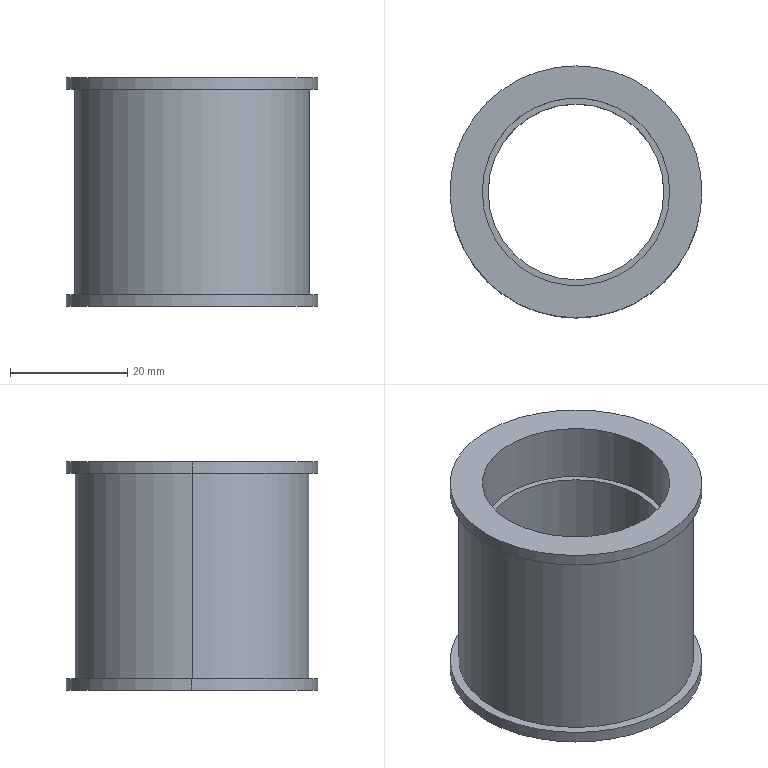Part | STEP file | Driven wheel | 1 solid | 18 faces | box 43 x 43 x 39 mm | volume 20276 mm3 | cylinder 12 | plane 6 | commonest cylinder face diameters 32 x4 43 x4 30 x2 40 x2
STEP:
#1=CARTESIAN_POINT('',(0.,0.,0.));
#2=DIRECTION('',(0.,0.,1.));
#3=DIRECTION('',(1.,0.,0.));
#4=AXIS2_PLACEMENT_3D('',#1,#2,#3);
#5=CARTESIAN_POINT('',(-20.,0.,35.));
#6=VERTEX_POINT('',#5);
#7=CARTESIAN_POINT('',(20.,0.,35.));
#8=VERTEX_POINT('',#7);
#9=CARTESIAN_POINT('',(0.,0.,35.));
#10=DIRECTION('',(0.,0.,-1.));
#11=DIRECTION('',(-1.,0.,0.));
#12=AXIS2_PLACEMENT_3D('',#9,#10,#11);
#13=CIRCLE('',#12,20.);
#14=CARTESIAN_POINT('',(0.,0.,35.));
#15=DIRECTION('',(0.,0.,-1.));
#16=DIRECTION('',(-1.,0.,0.));
#17=AXIS2_PLACEMENT_3D('',#14,#15,#16);
#18=CYLINDRICAL_SURFACE('',#17,20.);
#19=CARTESIAN_POINT('',(0.,0.));
#20=DIRECTION('',(1.,0.));
#21=VECTOR('',#20,1.);
#22=LINE('',#19,#21);
#23=(GEOMETRIC_REPRESENTATION_CONTEXT(2)PARAMETRIC_REPRESENTATION_CONTEXT()REPRESENTATION_CONTEXT('',''));
#24=DEFINITIONAL_REPRESENTATION('',(#22),#23);
#25=PCURVE('',#18,#24);
#26=CARTESIAN_POINT('',(0.,0.,35.));
#27=DIRECTION('',(0.,0.,1.));
#28=DIRECTION('',(1.,0.,0.));
#29=AXIS2_PLACEMENT_3D('',#26,#27,#28);
#30=PLANE('',#29);
#31=CARTESIAN_POINT('',(-20.,0.));
#32=CARTESIAN_POINT('',(-20.,34.641));
#33=CARTESIAN_POINT('',(10.,17.321));
#34=CARTESIAN_POINT('',(40.,0.));
#35=CARTESIAN_POINT('',(10.,-17.321));
#36=CARTESIAN_POINT('',(-20.,-34.641));
#37=CARTESIAN_POINT('',(-20.,0.));
#38=(BOUNDED_CURVE()B_SPLINE_CURVE(2,(#31,#32,#33,#34,#35,#36,#37),.UNSPECIFIED.,.T.,.F.)B_SPLINE_CURVE_WITH_KNOTS((1,2,2,2,2,1),(-2.094,0.,2.094,4.189,6.283,8.378),.UNSPECIFIED.)CURVE()GEOMETRIC_REPRESENTATION_ITEM()RATIONAL_B_SPLINE_CURVE((1.,0.5,1.,0.5,1.,0.5,1.))REPRESENTATION_ITEM(''));
#39=(GEOMETRIC_REPRESENTATION_CONTEXT(2)PARAMETRIC_REPRESENTATION_CONTEXT()REPRESENTATION_CONTEXT('',''));
#40=DEFINITIONAL_REPRESENTATION('',(#38),#39);
#41=PCURVE('',#30,#40);
#42=SURFACE_CURVE('',#13,(#25,#41),.PCURVE_S1.);
#43=EDGE_CURVE('',#6,#8,#42,.T.);
#44=ORIENTED_EDGE('',*,*,#43,.T.);
#45=CARTESIAN_POINT('',(20.,0.,0.));
#46=VERTEX_POINT('',#45);
#47=CARTESIAN_POINT('',(20.,0.,35.));
#48=DIRECTION('',(0.,0.,-1.));
#49=VECTOR('',#48,1.);
#50=LINE('',#47,#49);
#51=CARTESIAN_POINT('',(3.142,0.));
#52=DIRECTION('',(0.,1.));
#53=VECTOR('',#52,1.);
#54=LINE('',#51,#53);
#55=(GEOMETRIC_REPRESENTATION_CONTEXT(2)PARAMETRIC_REPRESENTATION_CONTEXT()REPRESENTATION_CONTEXT('',''));
#56=DEFINITIONAL_REPRESENTATION('',(#54),#55);
#57=PCURVE('',#18,#56);
#58=CARTESIAN_POINT('',(0.,0.,35.));
#59=DIRECTION('',(0.,0.,-1.));
#60=DIRECTION('',(-1.,0.,0.));
#61=AXIS2_PLACEMENT_3D('',#58,#59,#60);
#62=CYLINDRICAL_SURFACE('',#61,20.);
#63=CARTESIAN_POINT('',(3.142,0.));
#64=DIRECTION('',(0.,1.));
#65=VECTOR('',#64,1.);
#66=LINE('',#63,#65);
#67=(GEOMETRIC_REPRESENTATION_CONTEXT(2)PARAMETRIC_REPRESENTATION_CONTEXT()REPRESENTATION_CONTEXT('',''));
#68=DEFINITIONAL_REPRESENTATION('',(#66),#67);
#69=PCURVE('',#62,#68);
#70=SURFACE_CURVE('',#50,(#57,#69),.PCURVE_S1.);
#71=EDGE_CURVE('',#8,#46,#70,.T.);
#72=ORIENTED_EDGE('',*,*,#71,.T.);
#73=CARTESIAN_POINT('',(-20.,0.,0.));
#74=VERTEX_POINT('',#73);
#75=CARTESIAN_POINT('',(0.,0.,0.));
#76=DIRECTION('',(0.,0.,1.));
#77=DIRECTION('',(-1.,0.,0.));
#78=AXIS2_PLACEMENT_3D('',#75,#76,#77);
#79=CIRCLE('',#78,20.);
#80=CARTESIAN_POINT('',(6.283,35.));
#81=DIRECTION('',(-1.,0.));
#82=VECTOR('',#81,1.);
#83=LINE('',#80,#82);
#84=(GEOMETRIC_REPRESENTATION_CONTEXT(2)PARAMETRIC_REPRESENTATION_CONTEXT()REPRESENTATION_CONTEXT('',''));
#85=DEFINITIONAL_REPRESENTATION('',(#83),#84);
#86=PCURVE('',#18,#85);
#87=CARTESIAN_POINT('',(0.,0.,0.));
#88=DIRECTION('',(0.,0.,-1.));
#89=DIRECTION('',(-1.,0.,0.));
#90=AXIS2_PLACEMENT_3D('',#87,#88,#89);
#91=PLANE('',#90);
#92=CARTESIAN_POINT('',(20.,0.));
#93=CARTESIAN_POINT('',(20.,-34.641));
#94=CARTESIAN_POINT('',(-10.,-17.321));
#95=CARTESIAN_POINT('',(-40.,0.));
#96=CARTESIAN_POINT('',(-10.,17.321));
#97=CARTESIAN_POINT('',(20.,34.641));
#98=CARTESIAN_POINT('',(20.,0.));
#99=(BOUNDED_CURVE()B_SPLINE_CURVE(2,(#92,#93,#94,#95,#96,#97,#98),.UNSPECIFIED.,.T.,.F.)B_SPLINE_CURVE_WITH_KNOTS((1,2,2,2,2,1),(-2.094,0.,2.094,4.189,6.283,8.378),.UNSPECIFIED.)CURVE()GEOMETRIC_REPRESENTATION_ITEM()RATIONAL_B_SPLINE_CURVE((1.,0.5,1.,0.5,1.,0.5,1.))REPRESENTATION_ITEM(''));
#100=(GEOMETRIC_REPRESENTATION_CONTEXT(2)PARAMETRIC_REPRESENTATION_CONTEXT()REPRESENTATION_CONTEXT('',''));
#101=DEFINITIONAL_REPRESENTATION('',(#99),#100);
#102=PCURVE('',#91,#101);
#103=SURFACE_CURVE('',#79,(#86,#102),.PCURVE_S1.);
#104=EDGE_CURVE('',#46,#74,#103,.T.);
#105=ORIENTED_EDGE('',*,*,#104,.T.);
#106=CARTESIAN_POINT('',(-20.,0.,35.));
#107=DIRECTION('',(0.,0.,-1.));
#108=VECTOR('',#107,1.);
#109=LINE('',#106,#108);
#110=CARTESIAN_POINT('',(0.,0.));
#111=DIRECTION('',(0.,1.));
#112=VECTOR('',#111,1.);
#113=LINE('',#110,#112);
#114=(GEOMETRIC_REPRESENTATION_CONTEXT(2)PARAMETRIC_REPRESENTATION_CONTEXT()REPRESENTATION_CONTEXT('',''));
#115=DEFINITIONAL_REPRESENTATION('',(#113),#114);
#116=PCURVE('',#18,#115);
#117=CARTESIAN_POINT('',(6.283,0.));
#118=DIRECTION('',(0.,1.));
#119=VECTOR('',#118,1.);
#120=LINE('',#117,#119);
#121=(GEOMETRIC_REPRESENTATION_CONTEXT(2)PARAMETRIC_REPRESENTATION_CONTEXT()REPRESENTATION_CONTEXT('',''));
#122=DEFINITIONAL_REPRESENTATION('',(#120),#121);
#123=PCURVE('',#62,#122);
#124=SURFACE_CURVE('',#109,(#116,#123),.PCURVE_S1.);
#125=EDGE_CURVE('',#6,#74,#124,.T.);
#126=ORIENTED_EDGE('',*,*,#125,.F.);
#127=EDGE_LOOP('',(#44,#72,#105,#126));
#128=FACE_BOUND('',#127,.T.);
#129=ADVANCED_FACE('',(#128),#18,.T.);
#130=CARTESIAN_POINT('',(21.5,0.,-2.));
#131=VERTEX_POINT('',#130);
#132=CARTESIAN_POINT('',(-21.5,0.,-2.));
#133=VERTEX_POINT('',#132);
#134=CARTESIAN_POINT('',(0.,0.,-2.));
#135=DIRECTION('',(0.,0.,1.));
#136=DIRECTION('',(1.,0.,0.));
#137=AXIS2_PLACEMENT_3D('',#134,#135,#136);
#138=CIRCLE('',#137,21.5);
#139=CARTESIAN_POINT('',(0.,0.,-2.));
#140=DIRECTION('',(0.,0.,1.));
#141=DIRECTION('',(1.,0.,0.));
#142=AXIS2_PLACEMENT_3D('',#139,#140,#141);
#143=CYLINDRICAL_SURFACE('',#142,21.5);
#144=CARTESIAN_POINT('',(0.,0.));
#145=DIRECTION('',(1.,0.));
#146=VECTOR('',#145,1.);
#147=LINE('',#144,#146);
#148=(GEOMETRIC_REPRESENTATION_CONTEXT(2)PARAMETRIC_REPRESENTATION_CONTEXT()REPRESENTATION_CONTEXT('',''));
#149=DEFINITIONAL_REPRESENTATION('',(#147),#148);
#150=PCURVE('',#143,#149);
#151=CARTESIAN_POINT('',(0.,0.,-2.));
#152=DIRECTION('',(0.,0.,-1.));
#153=DIRECTION('',(-1.,0.,0.));
#154=AXIS2_PLACEMENT_3D('',#151,#152,#153);
#155=PLANE('',#154);
#156=CARTESIAN_POINT('',(-21.5,0.));
#157=CARTESIAN_POINT('',(-21.5,37.239));
#158=CARTESIAN_POINT('',(10.75,18.62));
#159=CARTESIAN_POINT('',(43.,0.));
#160=CARTESIAN_POINT('',(10.75,-18.62));
#161=CARTESIAN_POINT('',(-21.5,-37.239));
#162=CARTESIAN_POINT('',(-21.5,0.));
#163=(BOUNDED_CURVE()B_SPLINE_CURVE(2,(#156,#157,#158,#159,#160,#161,#162),.UNSPECIFIED.,.T.,.F.)B_SPLINE_CURVE_WITH_KNOTS((1,2,2,2,2,1),(-2.094,0.,2.094,4.189,6.283,8.378),.UNSPECIFIED.)CURVE()GEOMETRIC_REPRESENTATION_ITEM()RATIONAL_B_SPLINE_CURVE((1.,0.5,1.,0.5,1.,0.5,1.))REPRESENTATION_ITEM(''));
#164=(GEOMETRIC_REPRESENTATION_CONTEXT(2)PARAMETRIC_REPRESENTATION_CONTEXT()REPRESENTATION_CONTEXT('',''));
#165=DEFINITIONAL_REPRESENTATION('',(#163),#164);
#166=PCURVE('',#155,#165);
#167=SURFACE_CURVE('',#138,(#150,#166),.PCURVE_S1.);
#168=EDGE_CURVE('',#131,#133,#167,.T.);
#169=ORIENTED_EDGE('',*,*,#168,.T.);
#170=CARTESIAN_POINT('',(-21.5,0.,0.));
#171=VERTEX_POINT('',#170);
#172=CARTESIAN_POINT('',(-21.5,0.,-2.));
#173=DIRECTION('',(0.,0.,1.));
#174=VECTOR('',#173,1.);
#175=LINE('',#172,#174);
#176=CARTESIAN_POINT('',(3.142,0.));
#177=DIRECTION('',(0.,1.));
#178=VECTOR('',#177,1.);
#179=LINE('',#176,#178);
#180=(GEOMETRIC_REPRESENTATION_CONTEXT(2)PARAMETRIC_REPRESENTATION_CONTEXT()REPRESENTATION_CONTEXT('',''));
#181=DEFINITIONAL_REPRESENTATION('',(#179),#180);
#182=PCURVE('',#143,#181);
#183=CARTESIAN_POINT('',(0.,0.,-2.));
#184=DIRECTION('',(0.,0.,1.));
#185=DIRECTION('',(1.,0.,0.));
#186=AXIS2_PLACEMENT_3D('',#183,#184,#185);
#187=CYLINDRICAL_SURFACE('',#186,21.5);
#188=CARTESIAN_POINT('',(3.142,0.));
#189=DIRECTION('',(0.,1.));
#190=VECTOR('',#189,1.);
#191=LINE('',#188,#190);
#192=(GEOMETRIC_REPRESENTATION_CONTEXT(2)PARAMETRIC_REPRESENTATION_CONTEXT()REPRESENTATION_CONTEXT('',''));
#193=DEFINITIONAL_REPRESENTATION('',(#191),#192);
#194=PCURVE('',#187,#193);
#195=SURFACE_CURVE('',#175,(#182,#194),.PCURVE_S1.);
#196=EDGE_CURVE('',#133,#171,#195,.T.);
#197=ORIENTED_EDGE('',*,*,#196,.T.);
#198=CARTESIAN_POINT('',(21.5,0.,0.));
#199=VERTEX_POINT('',#198);
#200=CARTESIAN_POINT('',(0.,0.,0.));
#201=DIRECTION('',(0.,0.,-1.));
#202=DIRECTION('',(1.,0.,0.));
#203=AXIS2_PLACEMENT_3D('',#200,#201,#202);
#204=CIRCLE('',#203,21.5);
#205=CARTESIAN_POINT('',(6.283,2.));
#206=DIRECTION('',(-1.,0.));
#207=VECTOR('',#206,1.);
#208=LINE('',#205,#207);
#209=(GEOMETRIC_REPRESENTATION_CONTEXT(2)PARAMETRIC_REPRESENTATION_CONTEXT()REPRESENTATION_CONTEXT('',''));
#210=DEFINITIONAL_REPRESENTATION('',(#208),#209);
#211=PCURVE('',#143,#210);
#212=CARTESIAN_POINT('',(0.,0.));
#213=DIRECTION('',(-1.,0.));
#214=AXIS2_PLACEMENT_2D('',#212,#213);
#215=CIRCLE('',#214,21.5);
#216=(GEOMETRIC_REPRESENTATION_CONTEXT(2)PARAMETRIC_REPRESENTATION_CONTEXT()REPRESENTATION_CONTEXT('',''));
#217=DEFINITIONAL_REPRESENTATION('',(#215),#216);
#218=PCURVE('',#91,#217);
#219=SURFACE_CURVE('',#204,(#211,#218),.PCURVE_S1.);
#220=EDGE_CURVE('',#171,#199,#219,.T.);
#221=ORIENTED_EDGE('',*,*,#220,.T.);
#222=CARTESIAN_POINT('',(21.5,0.,-2.));
#223=DIRECTION('',(0.,0.,1.));
#224=VECTOR('',#223,1.);
#225=LINE('',#222,#224);
#226=CARTESIAN_POINT('',(0.,0.));
#227=DIRECTION('',(0.,1.));
#228=VECTOR('',#227,1.);
#229=LINE('',#226,#228);
#230=(GEOMETRIC_REPRESENTATION_CONTEXT(2)PARAMETRIC_REPRESENTATION_CONTEXT()REPRESENTATION_CONTEXT('',''));
#231=DEFINITIONAL_REPRESENTATION('',(#229),#230);
#232=PCURVE('',#143,#231);
#233=CARTESIAN_POINT('',(6.283,0.));
#234=DIRECTION('',(0.,1.));
#235=VECTOR('',#234,1.);
#236=LINE('',#233,#235);
#237=(GEOMETRIC_REPRESENTATION_CONTEXT(2)PARAMETRIC_REPRESENTATION_CONTEXT()REPRESENTATION_CONTEXT('',''));
#238=DEFINITIONAL_REPRESENTATION('',(#236),#237);
#239=PCURVE('',#187,#238);
#240=SURFACE_CURVE('',#225,(#232,#239),.PCURVE_S1.);
#241=EDGE_CURVE('',#131,#199,#240,.T.);
#242=ORIENTED_EDGE('',*,*,#241,.F.);
#243=EDGE_LOOP('',(#169,#197,#221,#242));
#244=FACE_BOUND('',#243,.T.);
#245=ADVANCED_FACE('',(#244),#143,.T.);
#246=CARTESIAN_POINT('',(-21.5,0.,37.));
#247=VERTEX_POINT('',#246);
#248=CARTESIAN_POINT('',(21.5,0.,37.));
#249=VERTEX_POINT('',#248);
#250=CARTESIAN_POINT('',(0.,0.,37.));
#251=DIRECTION('',(0.,0.,-1.));
#252=DIRECTION('',(-1.,0.,0.));
#253=AXIS2_PLACEMENT_3D('',#250,#251,#252);
#254=CIRCLE('',#253,21.5);
#255=CARTESIAN_POINT('',(0.,0.,37.));
#256=DIRECTION('',(0.,0.,-1.));
#257=DIRECTION('',(-1.,0.,0.));
#258=AXIS2_PLACEMENT_3D('',#255,#256,#257);
#259=CYLINDRICAL_SURFACE('',#258,21.5);
#260=CARTESIAN_POINT('',(0.,0.));
#261=DIRECTION('',(1.,0.));
#262=VECTOR('',#261,1.);
#263=LINE('',#260,#262);
#264=(GEOMETRIC_REPRESENTATION_CONTEXT(2)PARAMETRIC_REPRESENTATION_CONTEXT()REPRESENTATION_CONTEXT('',''));
#265=DEFINITIONAL_REPRESENTATION('',(#263),#264);
#266=PCURVE('',#259,#265);
#267=CARTESIAN_POINT('',(0.,0.,37.));
#268=DIRECTION('',(0.,0.,1.));
#269=DIRECTION('',(1.,0.,0.));
#270=AXIS2_PLACEMENT_3D('',#267,#268,#269);
#271=PLANE('',#270);
#272=CARTESIAN_POINT('',(-21.5,0.));
#273=CARTESIAN_POINT('',(-21.5,37.239));
#274=CARTESIAN_POINT('',(10.75,18.62));
#275=CARTESIAN_POINT('',(43.,0.));
#276=CARTESIAN_POINT('',(10.75,-18.62));
#277=CARTESIAN_POINT('',(-21.5,-37.239));
#278=CARTESIAN_POINT('',(-21.5,0.));
#279=(BOUNDED_CURVE()B_SPLINE_CURVE(2,(#272,#273,#274,#275,#276,#277,#278),.UNSPECIFIED.,.T.,.F.)B_SPLINE_CURVE_WITH_KNOTS((1,2,2,2,2,1),(-2.094,0.,2.094,4.189,6.283,8.378),.UNSPECIFIED.)CURVE()GEOMETRIC_REPRESENTATION_ITEM()RATIONAL_B_SPLINE_CURVE((1.,0.5,1.,0.5,1.,0.5,1.))REPRESENTATION_ITEM(''));
#280=(GEOMETRIC_REPRESENTATION_CONTEXT(2)PARAMETRIC_REPRESENTATION_CONTEXT()REPRESENTATION_CONTEXT('',''));
#281=DEFINITIONAL_REPRESENTATION('',(#279),#280);
#282=PCURVE('',#271,#281);
#283=SURFACE_CURVE('',#254,(#266,#282),.PCURVE_S1.);
#284=EDGE_CURVE('',#247,#249,#283,.T.);
#285=ORIENTED_EDGE('',*,*,#284,.T.);
#286=CARTESIAN_POINT('',(21.5,0.,35.));
#287=VERTEX_POINT('',#286);
#288=CARTESIAN_POINT('',(21.5,0.,37.));
#289=DIRECTION('',(0.,0.,-1.));
#290=VECTOR('',#289,1.);
#291=LINE('',#288,#290);
#292=CARTESIAN_POINT('',(3.142,0.));
#293=DIRECTION('',(0.,1.));
#294=VECTOR('',#293,1.);
#295=LINE('',#292,#294);
#296=(GEOMETRIC_REPRESENTATION_CONTEXT(2)PARAMETRIC_REPRESENTATION_CONTEXT()REPRESENTATION_CONTEXT('',''));
#297=DEFINITIONAL_REPRESENTATION('',(#295),#296);
#298=PCURVE('',#259,#297);
#299=CARTESIAN_POINT('',(0.,0.,37.));
#300=DIRECTION('',(0.,0.,-1.));
#301=DIRECTION('',(-1.,0.,0.));
#302=AXIS2_PLACEMENT_3D('',#299,#300,#301);
#303=CYLINDRICAL_SURFACE('',#302,21.5);
#304=CARTESIAN_POINT('',(3.142,0.));
#305=DIRECTION('',(0.,1.));
#306=VECTOR('',#305,1.);
#307=LINE('',#304,#306);
#308=(GEOMETRIC_REPRESENTATION_CONTEXT(2)PARAMETRIC_REPRESENTATION_CONTEXT()REPRESENTATION_CONTEXT('',''));
#309=DEFINITIONAL_REPRESENTATION('',(#307),#308);
#310=PCURVE('',#303,#309);
#311=SURFACE_CURVE('',#291,(#298,#310),.PCURVE_S1.);
#312=EDGE_CURVE('',#249,#287,#311,.T.);
#313=ORIENTED_EDGE('',*,*,#312,.T.);
#314=CARTESIAN_POINT('',(-21.5,0.,35.));
#315=VERTEX_POINT('',#314);
#316=CARTESIAN_POINT('',(0.,0.,35.));
#317=DIRECTION('',(0.,0.,1.));
#318=DIRECTION('',(-1.,0.,0.));
#319=AXIS2_PLACEMENT_3D('',#316,#317,#318);
#320=CIRCLE('',#319,21.5);
#321=CARTESIAN_POINT('',(6.283,2.));
#322=DIRECTION('',(-1.,0.));
#323=VECTOR('',#322,1.);
#324=LINE('',#321,#323);
#325=(GEOMETRIC_REPRESENTATION_CONTEXT(2)PARAMETRIC_REPRESENTATION_CONTEXT()REPRESENTATION_CONTEXT('',''));
#326=DEFINITIONAL_REPRESENTATION('',(#324),#325);
#327=PCURVE('',#259,#326);
#328=CARTESIAN_POINT('',(0.,0.));
#329=DIRECTION('',(-1.,0.));
#330=AXIS2_PLACEMENT_2D('',#328,#329);
#331=CIRCLE('',#330,21.5);
#332=(GEOMETRIC_REPRESENTATION_CONTEXT(2)PARAMETRIC_REPRESENTATION_CONTEXT()REPRESENTATION_CONTEXT('',''));
#333=DEFINITIONAL_REPRESENTATION('',(#331),#332);
#334=PCURVE('',#30,#333);
#335=SURFACE_CURVE('',#320,(#327,#334),.PCURVE_S1.);
#336=EDGE_CURVE('',#287,#315,#335,.T.);
#337=ORIENTED_EDGE('',*,*,#336,.T.);
#338=CARTESIAN_POINT('',(-21.5,0.,37.));
#339=DIRECTION('',(0.,0.,-1.));
#340=VECTOR('',#339,1.);
#341=LINE('',#338,#340);
#342=CARTESIAN_POINT('',(0.,0.));
#343=DIRECTION('',(0.,1.));
#344=VECTOR('',#343,1.);
#345=LINE('',#342,#344);
#346=(GEOMETRIC_REPRESENTATION_CONTEXT(2)PARAMETRIC_REPRESENTATION_CONTEXT()REPRESENTATION_CONTEXT('',''));
#347=DEFINITIONAL_REPRESENTATION('',(#345),#346);
#348=PCURVE('',#259,#347);
#349=CARTESIAN_POINT('',(6.283,0.));
#350=DIRECTION('',(0.,1.));
#351=VECTOR('',#350,1.);
#352=LINE('',#349,#351);
#353=(GEOMETRIC_REPRESENTATION_CONTEXT(2)PARAMETRIC_REPRESENTATION_CONTEXT()REPRESENTATION_CONTEXT('',''));
#354=DEFINITIONAL_REPRESENTATION('',(#352),#353);
#355=PCURVE('',#303,#354);
#356=SURFACE_CURVE('',#341,(#348,#355),.PCURVE_S1.);
#357=EDGE_CURVE('',#247,#315,#356,.T.);
#358=ORIENTED_EDGE('',*,*,#357,.F.);
#359=EDGE_LOOP('',(#285,#313,#337,#358));
#360=FACE_BOUND('',#359,.T.);
#361=ADVANCED_FACE('',(#360),#259,.T.);
#362=CARTESIAN_POINT('',(-16.,0.,8.));
#363=VERTEX_POINT('',#362);
#364=CARTESIAN_POINT('',(-16.,0.,-2.));
#365=VERTEX_POINT('',#364);
#366=CARTESIAN_POINT('',(-16.,0.,8.));
#367=DIRECTION('',(0.,0.,-1.));
#368=VECTOR('',#367,1.);
#369=LINE('',#366,#368);
#370=CARTESIAN_POINT('',(0.,0.,8.));
#371=DIRECTION('',(0.,0.,-1.));
#372=DIRECTION('',(-1.,0.,0.));
#373=AXIS2_PLACEMENT_3D('',#370,#371,#372);
#374=CYLINDRICAL_SURFACE('',#373,16.);
#375=CARTESIAN_POINT('',(6.283,0.));
#376=DIRECTION('',(0.,1.));
#377=VECTOR('',#376,1.);
#378=LINE('',#375,#377);
#379=(GEOMETRIC_REPRESENTATION_CONTEXT(2)PARAMETRIC_REPRESENTATION_CONTEXT()REPRESENTATION_CONTEXT('',''));
#380=DEFINITIONAL_REPRESENTATION('',(#378),#379);
#381=PCURVE('',#374,#380);
#382=CARTESIAN_POINT('',(0.,0.,8.));
#383=DIRECTION('',(0.,0.,-1.));
#384=DIRECTION('',(-1.,0.,0.));
#385=AXIS2_PLACEMENT_3D('',#382,#383,#384);
#386=CYLINDRICAL_SURFACE('',#385,16.);
#387=CARTESIAN_POINT('',(0.,0.));
#388=DIRECTION('',(0.,1.));
#389=VECTOR('',#388,1.);
#390=LINE('',#387,#389);
#391=(GEOMETRIC_REPRESENTATION_CONTEXT(2)PARAMETRIC_REPRESENTATION_CONTEXT()REPRESENTATION_CONTEXT('',''));
#392=DEFINITIONAL_REPRESENTATION('',(#390),#391);
#393=PCURVE('',#386,#392);
#394=SURFACE_CURVE('',#369,(#381,#393),.PCURVE_S1.);
#395=EDGE_CURVE('',#363,#365,#394,.T.);
#396=ORIENTED_EDGE('',*,*,#395,.T.);
#397=CARTESIAN_POINT('',(16.,0.,-2.));
#398=VERTEX_POINT('',#397);
#399=CARTESIAN_POINT('',(0.,0.,-2.));
#400=DIRECTION('',(0.,0.,1.));
#401=DIRECTION('',(-1.,0.,0.));
#402=AXIS2_PLACEMENT_3D('',#399,#400,#401);
#403=CIRCLE('',#402,16.);
#404=CARTESIAN_POINT('',(6.283,10.));
#405=DIRECTION('',(-1.,0.));
#406=VECTOR('',#405,1.);
#407=LINE('',#404,#406);
#408=(GEOMETRIC_REPRESENTATION_CONTEXT(2)PARAMETRIC_REPRESENTATION_CONTEXT()REPRESENTATION_CONTEXT('',''));
#409=DEFINITIONAL_REPRESENTATION('',(#407),#408);
#410=PCURVE('',#374,#409);
#411=CARTESIAN_POINT('',(16.,0.));
#412=CARTESIAN_POINT('',(16.,-27.713));
#413=CARTESIAN_POINT('',(-8.,-13.856));
#414=CARTESIAN_POINT('',(-32.,0.));
#415=CARTESIAN_POINT('',(-8.,13.856));
#416=CARTESIAN_POINT('',(16.,27.713));
#417=CARTESIAN_POINT('',(16.,0.));
#418=(BOUNDED_CURVE()B_SPLINE_CURVE(2,(#411,#412,#413,#414,#415,#416,#417),.UNSPECIFIED.,.T.,.F.)B_SPLINE_CURVE_WITH_KNOTS((1,2,2,2,2,1),(-2.094,0.,2.094,4.189,6.283,8.378),.UNSPECIFIED.)CURVE()GEOMETRIC_REPRESENTATION_ITEM()RATIONAL_B_SPLINE_CURVE((1.,0.5,1.,0.5,1.,0.5,1.))REPRESENTATION_ITEM(''));
#419=(GEOMETRIC_REPRESENTATION_CONTEXT(2)PARAMETRIC_REPRESENTATION_CONTEXT()REPRESENTATION_CONTEXT('',''));
#420=DEFINITIONAL_REPRESENTATION('',(#418),#419);
#421=PCURVE('',#155,#420);
#422=SURFACE_CURVE('',#403,(#410,#421),.PCURVE_S1.);
#423=EDGE_CURVE('',#365,#398,#422,.T.);
#424=ORIENTED_EDGE('',*,*,#423,.T.);
#425=CARTESIAN_POINT('',(16.,0.,8.));
#426=VERTEX_POINT('',#425);
#427=CARTESIAN_POINT('',(16.,0.,8.));
#428=DIRECTION('',(0.,0.,-1.));
#429=VECTOR('',#428,1.);
#430=LINE('',#427,#429);
#431=CARTESIAN_POINT('',(3.142,0.));
#432=DIRECTION('',(0.,1.));
#433=VECTOR('',#432,1.);
#434=LINE('',#431,#433);
#435=(GEOMETRIC_REPRESENTATION_CONTEXT(2)PARAMETRIC_REPRESENTATION_CONTEXT()REPRESENTATION_CONTEXT('',''));
#436=DEFINITIONAL_REPRESENTATION('',(#434),#435);
#437=PCURVE('',#374,#436);
#438=CARTESIAN_POINT('',(3.142,0.));
#439=DIRECTION('',(0.,1.));
#440=VECTOR('',#439,1.);
#441=LINE('',#438,#440);
#442=(GEOMETRIC_REPRESENTATION_CONTEXT(2)PARAMETRIC_REPRESENTATION_CONTEXT()REPRESENTATION_CONTEXT('',''));
#443=DEFINITIONAL_REPRESENTATION('',(#441),#442);
#444=PCURVE('',#386,#443);
#445=SURFACE_CURVE('',#430,(#437,#444),.PCURVE_S1.);
#446=EDGE_CURVE('',#426,#398,#445,.T.);
#447=ORIENTED_EDGE('',*,*,#446,.F.);
#448=CARTESIAN_POINT('',(0.,0.,8.));
#449=DIRECTION('',(0.,0.,-1.));
#450=DIRECTION('',(-1.,0.,0.));
#451=AXIS2_PLACEMENT_3D('',#448,#449,#450);
#452=CIRCLE('',#451,16.);
#453=CARTESIAN_POINT('',(0.,0.));
#454=DIRECTION('',(1.,0.));
#455=VECTOR('',#454,1.);
#456=LINE('',#453,#455);
#457=(GEOMETRIC_REPRESENTATION_CONTEXT(2)PARAMETRIC_REPRESENTATION_CONTEXT()REPRESENTATION_CONTEXT('',''));
#458=DEFINITIONAL_REPRESENTATION('',(#456),#457);
#459=PCURVE('',#374,#458);
#460=CARTESIAN_POINT('',(0.,0.,8.));
#461=DIRECTION('',(0.,0.,-1.));
#462=DIRECTION('',(-1.,0.,0.));
#463=AXIS2_PLACEMENT_3D('',#460,#461,#462);
#464=PLANE('',#463);
#465=CARTESIAN_POINT('',(0.,0.));
#466=DIRECTION('',(1.,0.));
#467=AXIS2_PLACEMENT_2D('',#465,#466);
#468=CIRCLE('',#467,16.);
#469=(GEOMETRIC_REPRESENTATION_CONTEXT(2)PARAMETRIC_REPRESENTATION_CONTEXT()REPRESENTATION_CONTEXT('',''));
#470=DEFINITIONAL_REPRESENTATION('',(#468),#469);
#471=PCURVE('',#464,#470);
#472=SURFACE_CURVE('',#452,(#459,#471),.PCURVE_S1.);
#473=EDGE_CURVE('',#426,#363,#472,.T.);
#474=ORIENTED_EDGE('',*,*,#473,.T.);
#475=EDGE_LOOP('',(#396,#424,#447,#474));
#476=FACE_BOUND('',#475,.F.);
#477=ADVANCED_FACE('',(#476),#374,.F.);
#478=CARTESIAN_POINT('',(16.,0.,27.));
#479=VERTEX_POINT('',#478);
#480=CARTESIAN_POINT('',(16.,0.,37.));
#481=VERTEX_POINT('',#480);
#482=CARTESIAN_POINT('',(16.,0.,27.));
#483=DIRECTION('',(0.,0.,1.));
#484=VECTOR('',#483,1.);
#485=LINE('',#482,#484);
#486=CARTESIAN_POINT('',(0.,0.,27.));
#487=DIRECTION('',(0.,0.,1.));
#488=DIRECTION('',(1.,0.,0.));
#489=AXIS2_PLACEMENT_3D('',#486,#487,#488);
#490=CYLINDRICAL_SURFACE('',#489,16.);
#491=CARTESIAN_POINT('',(6.283,0.));
#492=DIRECTION('',(0.,1.));
#493=VECTOR('',#492,1.);
#494=LINE('',#491,#493);
#495=(GEOMETRIC_REPRESENTATION_CONTEXT(2)PARAMETRIC_REPRESENTATION_CONTEXT()REPRESENTATION_CONTEXT('',''));
#496=DEFINITIONAL_REPRESENTATION('',(#494),#495);
#497=PCURVE('',#490,#496);
#498=CARTESIAN_POINT('',(0.,0.,27.));
#499=DIRECTION('',(0.,0.,1.));
#500=DIRECTION('',(1.,0.,0.));
#501=AXIS2_PLACEMENT_3D('',#498,#499,#500);
#502=CYLINDRICAL_SURFACE('',#501,16.);
#503=CARTESIAN_POINT('',(0.,0.));
#504=DIRECTION('',(0.,1.));
#505=VECTOR('',#504,1.);
#506=LINE('',#503,#505);
#507=(GEOMETRIC_REPRESENTATION_CONTEXT(2)PARAMETRIC_REPRESENTATION_CONTEXT()REPRESENTATION_CONTEXT('',''));
#508=DEFINITIONAL_REPRESENTATION('',(#506),#507);
#509=PCURVE('',#502,#508);
#510=SURFACE_CURVE('',#485,(#497,#509),.PCURVE_S1.);
#511=EDGE_CURVE('',#479,#481,#510,.T.);
#512=ORIENTED_EDGE('',*,*,#511,.T.);
#513=CARTESIAN_POINT('',(-16.,0.,37.));
#514=VERTEX_POINT('',#513);
#515=CARTESIAN_POINT('',(0.,0.,37.));
#516=DIRECTION('',(0.,0.,-1.));
#517=DIRECTION('',(1.,0.,0.));
#518=AXIS2_PLACEMENT_3D('',#515,#516,#517);
#519=CIRCLE('',#518,16.);
#520=CARTESIAN_POINT('',(6.283,10.));
#521=DIRECTION('',(-1.,0.));
#522=VECTOR('',#521,1.);
#523=LINE('',#520,#522);
#524=(GEOMETRIC_REPRESENTATION_CONTEXT(2)PARAMETRIC_REPRESENTATION_CONTEXT()REPRESENTATION_CONTEXT('',''));
#525=DEFINITIONAL_REPRESENTATION('',(#523),#524);
#526=PCURVE('',#490,#525);
#527=CARTESIAN_POINT('',(16.,0.));
#528=CARTESIAN_POINT('',(16.,-27.713));
#529=CARTESIAN_POINT('',(-8.,-13.856));
#530=CARTESIAN_POINT('',(-32.,0.));
#531=CARTESIAN_POINT('',(-8.,13.856));
#532=CARTESIAN_POINT('',(16.,27.713));
#533=CARTESIAN_POINT('',(16.,0.));
#534=(BOUNDED_CURVE()B_SPLINE_CURVE(2,(#527,#528,#529,#530,#531,#532,#533),.UNSPECIFIED.,.T.,.F.)B_SPLINE_CURVE_WITH_KNOTS((1,2,2,2,2,1),(-2.094,0.,2.094,4.189,6.283,8.378),.UNSPECIFIED.)CURVE()GEOMETRIC_REPRESENTATION_ITEM()RATIONAL_B_SPLINE_CURVE((1.,0.5,1.,0.5,1.,0.5,1.))REPRESENTATION_ITEM(''));
#535=(GEOMETRIC_REPRESENTATION_CONTEXT(2)PARAMETRIC_REPRESENTATION_CONTEXT()REPRESENTATION_CONTEXT('',''));
#536=DEFINITIONAL_REPRESENTATION('',(#534),#535);
#537=PCURVE('',#271,#536);
#538=SURFACE_CURVE('',#519,(#526,#537),.PCURVE_S1.);
#539=EDGE_CURVE('',#481,#514,#538,.T.);
#540=ORIENTED_EDGE('',*,*,#539,.T.);
#541=CARTESIAN_POINT('',(-16.,0.,27.));
#542=VERTEX_POINT('',#541);
#543=CARTESIAN_POINT('',(-16.,0.,27.));
#544=DIRECTION('',(0.,0.,1.));
#545=VECTOR('',#544,1.);
#546=LINE('',#543,#545);
#547=CARTESIAN_POINT('',(3.142,0.));
#548=DIRECTION('',(0.,1.));
#549=VECTOR('',#548,1.);
#550=LINE('',#547,#549);
#551=(GEOMETRIC_REPRESENTATION_CONTEXT(2)PARAMETRIC_REPRESENTATION_CONTEXT()REPRESENTATION_CONTEXT('',''));
#552=DEFINITIONAL_REPRESENTATION('',(#550),#551);
#553=PCURVE('',#490,#552);
#554=CARTESIAN_POINT('',(3.142,0.));
#555=DIRECTION('',(0.,1.));
#556=VECTOR('',#555,1.);
#557=LINE('',#554,#556);
#558=(GEOMETRIC_REPRESENTATION_CONTEXT(2)PARAMETRIC_REPRESENTATION_CONTEXT()REPRESENTATION_CONTEXT('',''));
#559=DEFINITIONAL_REPRESENTATION('',(#557),#558);
#560=PCURVE('',#502,#559);
#561=SURFACE_CURVE('',#546,(#553,#560),.PCURVE_S1.);
#562=EDGE_CURVE('',#542,#514,#561,.T.);
#563=ORIENTED_EDGE('',*,*,#562,.F.);
#564=CARTESIAN_POINT('',(0.,0.,27.));
#565=DIRECTION('',(0.,0.,1.));
#566=DIRECTION('',(1.,0.,0.));
#567=AXIS2_PLACEMENT_3D('',#564,#565,#566);
#568=CIRCLE('',#567,16.);
#569=CARTESIAN_POINT('',(0.,0.));
#570=DIRECTION('',(1.,0.));
#571=VECTOR('',#570,1.);
#572=LINE('',#569,#571);
#573=(GEOMETRIC_REPRESENTATION_CONTEXT(2)PARAMETRIC_REPRESENTATION_CONTEXT()REPRESENTATION_CONTEXT('',''));
#574=DEFINITIONAL_REPRESENTATION('',(#572),#573);
#575=PCURVE('',#490,#574);
#576=CARTESIAN_POINT('',(0.,0.,27.));
#577=DIRECTION('',(0.,0.,1.));
#578=DIRECTION('',(1.,0.,0.));
#579=AXIS2_PLACEMENT_3D('',#576,#577,#578);
#580=PLANE('',#579);
#581=CARTESIAN_POINT('',(0.,0.));
#582=DIRECTION('',(1.,0.));
#583=AXIS2_PLACEMENT_2D('',#581,#582);
#584=CIRCLE('',#583,16.);
#585=(GEOMETRIC_REPRESENTATION_CONTEXT(2)PARAMETRIC_REPRESENTATION_CONTEXT()REPRESENTATION_CONTEXT('',''));
#586=DEFINITIONAL_REPRESENTATION('',(#584),#585);
#587=PCURVE('',#580,#586);
#588=SURFACE_CURVE('',#568,(#575,#587),.PCURVE_S1.);
#589=EDGE_CURVE('',#542,#479,#588,.T.);
#590=ORIENTED_EDGE('',*,*,#589,.T.);
#591=EDGE_LOOP('',(#512,#540,#563,#590));
#592=FACE_BOUND('',#591,.F.);
#593=ADVANCED_FACE('',(#592),#490,.F.);
#594=CARTESIAN_POINT('',(15.,0.,8.));
#595=VERTEX_POINT('',#594);
#596=CARTESIAN_POINT('',(15.,0.,27.));
#597=VERTEX_POINT('',#596);
#598=CARTESIAN_POINT('',(15.,0.,-2.));
#599=DIRECTION('',(0.,0.,1.));
#600=VECTOR('',#599,1.);
#601=LINE('',#598,#600);
#602=CARTESIAN_POINT('',(0.,0.,-2.));
#603=DIRECTION('',(0.,0.,1.));
#604=DIRECTION('',(1.,0.,0.));
#605=AXIS2_PLACEMENT_3D('',#602,#603,#604);
#606=CYLINDRICAL_SURFACE('',#605,15.);
#607=CARTESIAN_POINT('',(6.283,0.));
#608=DIRECTION('',(0.,1.));
#609=VECTOR('',#608,1.);
#610=LINE('',#607,#609);
#611=(GEOMETRIC_REPRESENTATION_CONTEXT(2)PARAMETRIC_REPRESENTATION_CONTEXT()REPRESENTATION_CONTEXT('',''));
#612=DEFINITIONAL_REPRESENTATION('',(#610),#611);
#613=PCURVE('',#606,#612);
#614=CARTESIAN_POINT('',(0.,0.,-2.));
#615=DIRECTION('',(0.,0.,1.));
#616=DIRECTION('',(1.,0.,0.));
#617=AXIS2_PLACEMENT_3D('',#614,#615,#616);
#618=CYLINDRICAL_SURFACE('',#617,15.);
#619=CARTESIAN_POINT('',(0.,0.));
#620=DIRECTION('',(0.,1.));
#621=VECTOR('',#620,1.);
#622=LINE('',#619,#621);
#623=(GEOMETRIC_REPRESENTATION_CONTEXT(2)PARAMETRIC_REPRESENTATION_CONTEXT()REPRESENTATION_CONTEXT('',''));
#624=DEFINITIONAL_REPRESENTATION('',(#622),#623);
#625=PCURVE('',#618,#624);
#626=SURFACE_CURVE('',#601,(#613,#625),.PCURVE_S1.);
#627=EDGE_CURVE('',#595,#597,#626,.T.);
#628=ORIENTED_EDGE('',*,*,#627,.T.);
#629=CARTESIAN_POINT('',(-15.,0.,27.));
#630=VERTEX_POINT('',#629);
#631=CARTESIAN_POINT('',(0.,0.,27.));
#632=DIRECTION('',(0.,0.,-1.));
#633=DIRECTION('',(1.,0.,0.));
#634=AXIS2_PLACEMENT_3D('',#631,#632,#633);
#635=CIRCLE('',#634,15.);
#636=CARTESIAN_POINT('',(6.283,29.));
#637=DIRECTION('',(-1.,0.));
#638=VECTOR('',#637,1.);
#639=LINE('',#636,#638);
#640=(GEOMETRIC_REPRESENTATION_CONTEXT(2)PARAMETRIC_REPRESENTATION_CONTEXT()REPRESENTATION_CONTEXT('',''));
#641=DEFINITIONAL_REPRESENTATION('',(#639),#640);
#642=PCURVE('',#606,#641);
#643=CARTESIAN_POINT('',(15.,0.));
#644=CARTESIAN_POINT('',(15.,-25.981));
#645=CARTESIAN_POINT('',(-7.5,-12.99));
#646=CARTESIAN_POINT('',(-30.,0.));
#647=CARTESIAN_POINT('',(-7.5,12.99));
#648=CARTESIAN_POINT('',(15.,25.981));
#649=CARTESIAN_POINT('',(15.,0.));
#650=(BOUNDED_CURVE()B_SPLINE_CURVE(2,(#643,#644,#645,#646,#647,#648,#649),.UNSPECIFIED.,.T.,.F.)B_SPLINE_CURVE_WITH_KNOTS((1,2,2,2,2,1),(-2.094,0.,2.094,4.189,6.283,8.378),.UNSPECIFIED.)CURVE()GEOMETRIC_REPRESENTATION_ITEM()RATIONAL_B_SPLINE_CURVE((1.,0.5,1.,0.5,1.,0.5,1.))REPRESENTATION_ITEM(''));
#651=(GEOMETRIC_REPRESENTATION_CONTEXT(2)PARAMETRIC_REPRESENTATION_CONTEXT()REPRESENTATION_CONTEXT('',''));
#652=DEFINITIONAL_REPRESENTATION('',(#650),#651);
#653=PCURVE('',#580,#652);
#654=SURFACE_CURVE('',#635,(#642,#653),.PCURVE_S1.);
#655=EDGE_CURVE('',#597,#630,#654,.T.);
#656=ORIENTED_EDGE('',*,*,#655,.T.);
#657=CARTESIAN_POINT('',(-15.,0.,8.));
#658=VERTEX_POINT('',#657);
#659=CARTESIAN_POINT('',(-15.,0.,-2.));
#660=DIRECTION('',(0.,0.,1.));
#661=VECTOR('',#660,1.);
#662=LINE('',#659,#661);
#663=CARTESIAN_POINT('',(3.142,0.));
#664=DIRECTION('',(0.,1.));
#665=VECTOR('',#664,1.);
#666=LINE('',#663,#665);
#667=(GEOMETRIC_REPRESENTATION_CONTEXT(2)PARAMETRIC_REPRESENTATION_CONTEXT()REPRESENTATION_CONTEXT('',''));
#668=DEFINITIONAL_REPRESENTATION('',(#666),#667);
#669=PCURVE('',#606,#668);
#670=CARTESIAN_POINT('',(3.142,0.));
#671=DIRECTION('',(0.,1.));
#672=VECTOR('',#671,1.);
#673=LINE('',#670,#672);
#674=(GEOMETRIC_REPRESENTATION_CONTEXT(2)PARAMETRIC_REPRESENTATION_CONTEXT()REPRESENTATION_CONTEXT('',''));
#675=DEFINITIONAL_REPRESENTATION('',(#673),#674);
#676=PCURVE('',#618,#675);
#677=SURFACE_CURVE('',#662,(#669,#676),.PCURVE_S1.);
#678=EDGE_CURVE('',#658,#630,#677,.T.);
#679=ORIENTED_EDGE('',*,*,#678,.F.);
#680=CARTESIAN_POINT('',(0.,0.,8.));
#681=DIRECTION('',(0.,0.,1.));
#682=DIRECTION('',(1.,0.,0.));
#683=AXIS2_PLACEMENT_3D('',#680,#681,#682);
#684=CIRCLE('',#683,15.);
#685=CARTESIAN_POINT('',(0.,10.));
#686=DIRECTION('',(1.,0.));
#687=VECTOR('',#686,1.);
#688=LINE('',#685,#687);
#689=(GEOMETRIC_REPRESENTATION_CONTEXT(2)PARAMETRIC_REPRESENTATION_CONTEXT()REPRESENTATION_CONTEXT('',''));
#690=DEFINITIONAL_REPRESENTATION('',(#688),#689);
#691=PCURVE('',#606,#690);
#692=CARTESIAN_POINT('',(-15.,0.));
#693=CARTESIAN_POINT('',(-15.,25.981));
#694=CARTESIAN_POINT('',(7.5,12.99));
#695=CARTESIAN_POINT('',(30.,0.));
#696=CARTESIAN_POINT('',(7.5,-12.99));
#697=CARTESIAN_POINT('',(-15.,-25.981));
#698=CARTESIAN_POINT('',(-15.,0.));
#699=(BOUNDED_CURVE()B_SPLINE_CURVE(2,(#692,#693,#694,#695,#696,#697,#698),.UNSPECIFIED.,.T.,.F.)B_SPLINE_CURVE_WITH_KNOTS((1,2,2,2,2,1),(-2.094,0.,2.094,4.189,6.283,8.378),.UNSPECIFIED.)CURVE()GEOMETRIC_REPRESENTATION_ITEM()RATIONAL_B_SPLINE_CURVE((1.,0.5,1.,0.5,1.,0.5,1.))REPRESENTATION_ITEM(''));
#700=(GEOMETRIC_REPRESENTATION_CONTEXT(2)PARAMETRIC_REPRESENTATION_CONTEXT()REPRESENTATION_CONTEXT('',''));
#701=DEFINITIONAL_REPRESENTATION('',(#699),#700);
#702=PCURVE('',#464,#701);
#703=SURFACE_CURVE('',#684,(#691,#702),.PCURVE_S1.);
#704=EDGE_CURVE('',#658,#595,#703,.T.);
#705=ORIENTED_EDGE('',*,*,#704,.T.);
#706=EDGE_LOOP('',(#628,#656,#679,#705));
#707=FACE_BOUND('',#706,.F.);
#708=ADVANCED_FACE('',(#707),#606,.F.);
#709=ORIENTED_EDGE('',*,*,#71,.F.);
#710=CARTESIAN_POINT('',(0.,0.,35.));
#711=DIRECTION('',(0.,0.,-1.));
#712=DIRECTION('',(-1.,0.,0.));
#713=AXIS2_PLACEMENT_3D('',#710,#711,#712);
#714=CIRCLE('',#713,20.);
#715=CARTESIAN_POINT('',(0.,0.));
#716=DIRECTION('',(1.,0.));
#717=VECTOR('',#716,1.);
#718=LINE('',#715,#717);
#719=(GEOMETRIC_REPRESENTATION_CONTEXT(2)PARAMETRIC_REPRESENTATION_CONTEXT()REPRESENTATION_CONTEXT('',''));
#720=DEFINITIONAL_REPRESENTATION('',(#718),#719);
#721=PCURVE('',#62,#720);
#722=CARTESIAN_POINT('',(-20.,0.));
#723=CARTESIAN_POINT('',(-20.,34.641));
#724=CARTESIAN_POINT('',(10.,17.321));
#725=CARTESIAN_POINT('',(40.,0.));
#726=CARTESIAN_POINT('',(10.,-17.321));
#727=CARTESIAN_POINT('',(-20.,-34.641));
#728=CARTESIAN_POINT('',(-20.,0.));
#729=(BOUNDED_CURVE()B_SPLINE_CURVE(2,(#722,#723,#724,#725,#726,#727,#728),.UNSPECIFIED.,.T.,.F.)B_SPLINE_CURVE_WITH_KNOTS((1,2,2,2,2,1),(-2.094,0.,2.094,4.189,6.283,8.378),.UNSPECIFIED.)CURVE()GEOMETRIC_REPRESENTATION_ITEM()RATIONAL_B_SPLINE_CURVE((1.,0.5,1.,0.5,1.,0.5,1.))REPRESENTATION_ITEM(''));
#730=(GEOMETRIC_REPRESENTATION_CONTEXT(2)PARAMETRIC_REPRESENTATION_CONTEXT()REPRESENTATION_CONTEXT('',''));
#731=DEFINITIONAL_REPRESENTATION('',(#729),#730);
#732=PCURVE('',#30,#731);
#733=SURFACE_CURVE('',#714,(#721,#732),.PCURVE_S1.);
#734=EDGE_CURVE('',#8,#6,#733,.T.);
#735=ORIENTED_EDGE('',*,*,#734,.T.);
#736=ORIENTED_EDGE('',*,*,#125,.T.);
#737=CARTESIAN_POINT('',(0.,0.,0.));
#738=DIRECTION('',(0.,0.,1.));
#739=DIRECTION('',(-1.,0.,0.));
#740=AXIS2_PLACEMENT_3D('',#737,#738,#739);
#741=CIRCLE('',#740,20.);
#742=CARTESIAN_POINT('',(6.283,35.));
#743=DIRECTION('',(-1.,0.));
#744=VECTOR('',#743,1.);
#745=LINE('',#742,#744);
#746=(GEOMETRIC_REPRESENTATION_CONTEXT(2)PARAMETRIC_REPRESENTATION_CONTEXT()REPRESENTATION_CONTEXT('',''));
#747=DEFINITIONAL_REPRESENTATION('',(#745),#746);
#748=PCURVE('',#62,#747);
#749=CARTESIAN_POINT('',(20.,0.));
#750=CARTESIAN_POINT('',(20.,-34.641));
#751=CARTESIAN_POINT('',(-10.,-17.321));
#752=CARTESIAN_POINT('',(-40.,0.));
#753=CARTESIAN_POINT('',(-10.,17.321));
#754=CARTESIAN_POINT('',(20.,34.641));
#755=CARTESIAN_POINT('',(20.,0.));
#756=(BOUNDED_CURVE()B_SPLINE_CURVE(2,(#749,#750,#751,#752,#753,#754,#755),.UNSPECIFIED.,.T.,.F.)B_SPLINE_CURVE_WITH_KNOTS((1,2,2,2,2,1),(-2.094,0.,2.094,4.189,6.283,8.378),.UNSPECIFIED.)CURVE()GEOMETRIC_REPRESENTATION_ITEM()RATIONAL_B_SPLINE_CURVE((1.,0.5,1.,0.5,1.,0.5,1.))REPRESENTATION_ITEM(''));
#757=(GEOMETRIC_REPRESENTATION_CONTEXT(2)PARAMETRIC_REPRESENTATION_CONTEXT()REPRESENTATION_CONTEXT('',''));
#758=DEFINITIONAL_REPRESENTATION('',(#756),#757);
#759=PCURVE('',#91,#758);
#760=SURFACE_CURVE('',#741,(#748,#759),.PCURVE_S1.);
#761=EDGE_CURVE('',#74,#46,#760,.T.);
#762=ORIENTED_EDGE('',*,*,#761,.T.);
#763=EDGE_LOOP('',(#709,#735,#736,#762));
#764=FACE_BOUND('',#763,.T.);
#765=ADVANCED_FACE('',(#764),#62,.T.);
#766=ORIENTED_EDGE('',*,*,#761,.F.);
#767=ORIENTED_EDGE('',*,*,#104,.F.);
#768=EDGE_LOOP('',(#766,#767));
#769=FACE_BOUND('',#768,.T.);
#770=CARTESIAN_POINT('',(0.,0.,0.));
#771=DIRECTION('',(0.,0.,-1.));
#772=DIRECTION('',(1.,0.,0.));
#773=AXIS2_PLACEMENT_3D('',#770,#771,#772);
#774=CIRCLE('',#773,21.5);
#775=CARTESIAN_POINT('',(0.,0.));
#776=DIRECTION('',(-1.,0.));
#777=AXIS2_PLACEMENT_2D('',#775,#776);
#778=CIRCLE('',#777,21.5);
#779=(GEOMETRIC_REPRESENTATION_CONTEXT(2)PARAMETRIC_REPRESENTATION_CONTEXT()REPRESENTATION_CONTEXT('',''));
#780=DEFINITIONAL_REPRESENTATION('',(#778),#779);
#781=PCURVE('',#91,#780);
#782=CARTESIAN_POINT('',(6.283,2.));
#783=DIRECTION('',(-1.,0.));
#784=VECTOR('',#783,1.);
#785=LINE('',#782,#784);
#786=(GEOMETRIC_REPRESENTATION_CONTEXT(2)PARAMETRIC_REPRESENTATION_CONTEXT()REPRESENTATION_CONTEXT('',''));
#787=DEFINITIONAL_REPRESENTATION('',(#785),#786);
#788=PCURVE('',#187,#787);
#789=SURFACE_CURVE('',#774,(#781,#788),.PCURVE_S1.);
#790=EDGE_CURVE('',#199,#171,#789,.T.);
#791=ORIENTED_EDGE('',*,*,#790,.F.);
#792=ORIENTED_EDGE('',*,*,#220,.F.);
#793=EDGE_LOOP('',(#791,#792));
#794=FACE_BOUND('',#793,.T.);
#795=ADVANCED_FACE('',(#769,#794),#91,.F.);
#796=ORIENTED_EDGE('',*,*,#43,.F.);
#797=ORIENTED_EDGE('',*,*,#734,.F.);
#798=EDGE_LOOP('',(#796,#797));
#799=FACE_BOUND('',#798,.T.);
#800=CARTESIAN_POINT('',(0.,0.,35.));
#801=DIRECTION('',(0.,0.,1.));
#802=DIRECTION('',(-1.,0.,0.));
#803=AXIS2_PLACEMENT_3D('',#800,#801,#802);
#804=CIRCLE('',#803,21.5);
#805=CARTESIAN_POINT('',(0.,0.));
#806=DIRECTION('',(-1.,0.));
#807=AXIS2_PLACEMENT_2D('',#805,#806);
#808=CIRCLE('',#807,21.5);
#809=(GEOMETRIC_REPRESENTATION_CONTEXT(2)PARAMETRIC_REPRESENTATION_CONTEXT()REPRESENTATION_CONTEXT('',''));
#810=DEFINITIONAL_REPRESENTATION('',(#808),#809);
#811=PCURVE('',#30,#810);
#812=CARTESIAN_POINT('',(6.283,2.));
#813=DIRECTION('',(-1.,0.));
#814=VECTOR('',#813,1.);
#815=LINE('',#812,#814);
#816=(GEOMETRIC_REPRESENTATION_CONTEXT(2)PARAMETRIC_REPRESENTATION_CONTEXT()REPRESENTATION_CONTEXT('',''));
#817=DEFINITIONAL_REPRESENTATION('',(#815),#816);
#818=PCURVE('',#303,#817);
#819=SURFACE_CURVE('',#804,(#811,#818),.PCURVE_S1.);
#820=EDGE_CURVE('',#315,#287,#819,.T.);
#821=ORIENTED_EDGE('',*,*,#820,.F.);
#822=ORIENTED_EDGE('',*,*,#336,.F.);
#823=EDGE_LOOP('',(#821,#822));
#824=FACE_BOUND('',#823,.T.);
#825=ADVANCED_FACE('',(#799,#824),#30,.F.);
#826=ORIENTED_EDGE('',*,*,#196,.F.);
#827=CARTESIAN_POINT('',(0.,0.,-2.));
#828=DIRECTION('',(0.,0.,1.));
#829=DIRECTION('',(1.,0.,0.));
#830=AXIS2_PLACEMENT_3D('',#827,#828,#829);
#831=CIRCLE('',#830,21.5);
#832=CARTESIAN_POINT('',(0.,0.));
#833=DIRECTION('',(1.,0.));
#834=VECTOR('',#833,1.);
#835=LINE('',#832,#834);
#836=(GEOMETRIC_REPRESENTATION_CONTEXT(2)PARAMETRIC_REPRESENTATION_CONTEXT()REPRESENTATION_CONTEXT('',''));
#837=DEFINITIONAL_REPRESENTATION('',(#835),#836);
#838=PCURVE('',#187,#837);
#839=CARTESIAN_POINT('',(-21.5,0.));
#840=CARTESIAN_POINT('',(-21.5,37.239));
#841=CARTESIAN_POINT('',(10.75,18.62));
#842=CARTESIAN_POINT('',(43.,0.));
#843=CARTESIAN_POINT('',(10.75,-18.62));
#844=CARTESIAN_POINT('',(-21.5,-37.239));
#845=CARTESIAN_POINT('',(-21.5,0.));
#846=(BOUNDED_CURVE()B_SPLINE_CURVE(2,(#839,#840,#841,#842,#843,#844,#845),.UNSPECIFIED.,.T.,.F.)B_SPLINE_CURVE_WITH_KNOTS((1,2,2,2,2,1),(-2.094,0.,2.094,4.189,6.283,8.378),.UNSPECIFIED.)CURVE()GEOMETRIC_REPRESENTATION_ITEM()RATIONAL_B_SPLINE_CURVE((1.,0.5,1.,0.5,1.,0.5,1.))REPRESENTATION_ITEM(''));
#847=(GEOMETRIC_REPRESENTATION_CONTEXT(2)PARAMETRIC_REPRESENTATION_CONTEXT()REPRESENTATION_CONTEXT('',''));
#848=DEFINITIONAL_REPRESENTATION('',(#846),#847);
#849=PCURVE('',#155,#848);
#850=SURFACE_CURVE('',#831,(#838,#849),.PCURVE_S1.);
#851=EDGE_CURVE('',#133,#131,#850,.T.);
#852=ORIENTED_EDGE('',*,*,#851,.T.);
#853=ORIENTED_EDGE('',*,*,#241,.T.);
#854=ORIENTED_EDGE('',*,*,#790,.T.);
#855=EDGE_LOOP('',(#826,#852,#853,#854));
#856=FACE_BOUND('',#855,.T.);
#857=ADVANCED_FACE('',(#856),#187,.T.);
#858=ORIENTED_EDGE('',*,*,#312,.F.);
#859=CARTESIAN_POINT('',(0.,0.,37.));
#860=DIRECTION('',(0.,0.,-1.));
#861=DIRECTION('',(-1.,0.,0.));
#862=AXIS2_PLACEMENT_3D('',#859,#860,#861);
#863=CIRCLE('',#862,21.5);
#864=CARTESIAN_POINT('',(0.,0.));
#865=DIRECTION('',(1.,0.));
#866=VECTOR('',#865,1.);
#867=LINE('',#864,#866);
#868=(GEOMETRIC_REPRESENTATION_CONTEXT(2)PARAMETRIC_REPRESENTATION_CONTEXT()REPRESENTATION_CONTEXT('',''));
#869=DEFINITIONAL_REPRESENTATION('',(#867),#868);
#870=PCURVE('',#303,#869);
#871=CARTESIAN_POINT('',(-21.5,0.));
#872=CARTESIAN_POINT('',(-21.5,37.239));
#873=CARTESIAN_POINT('',(10.75,18.62));
#874=CARTESIAN_POINT('',(43.,0.));
#875=CARTESIAN_POINT('',(10.75,-18.62));
#876=CARTESIAN_POINT('',(-21.5,-37.239));
#877=CARTESIAN_POINT('',(-21.5,0.));
#878=(BOUNDED_CURVE()B_SPLINE_CURVE(2,(#871,#872,#873,#874,#875,#876,#877),.UNSPECIFIED.,.T.,.F.)B_SPLINE_CURVE_WITH_KNOTS((1,2,2,2,2,1),(-2.094,0.,2.094,4.189,6.283,8.378),.UNSPECIFIED.)CURVE()GEOMETRIC_REPRESENTATION_ITEM()RATIONAL_B_SPLINE_CURVE((1.,0.5,1.,0.5,1.,0.5,1.))REPRESENTATION_ITEM(''));
#879=(GEOMETRIC_REPRESENTATION_CONTEXT(2)PARAMETRIC_REPRESENTATION_CONTEXT()REPRESENTATION_CONTEXT('',''));
#880=DEFINITIONAL_REPRESENTATION('',(#878),#879);
#881=PCURVE('',#271,#880);
#882=SURFACE_CURVE('',#863,(#870,#881),.PCURVE_S1.);
#883=EDGE_CURVE('',#249,#247,#882,.T.);
#884=ORIENTED_EDGE('',*,*,#883,.T.);
#885=ORIENTED_EDGE('',*,*,#357,.T.);
#886=ORIENTED_EDGE('',*,*,#820,.T.);
#887=EDGE_LOOP('',(#858,#884,#885,#886));
#888=FACE_BOUND('',#887,.T.);
#889=ADVANCED_FACE('',(#888),#303,.T.);
#890=ORIENTED_EDGE('',*,*,#168,.F.);
#891=ORIENTED_EDGE('',*,*,#851,.F.);
#892=EDGE_LOOP('',(#890,#891));
#893=FACE_BOUND('',#892,.T.);
#894=ORIENTED_EDGE('',*,*,#423,.T.);
#895=CARTESIAN_POINT('',(0.,0.,-2.));
#896=DIRECTION('',(0.,0.,1.));
#897=DIRECTION('',(-1.,0.,0.));
#898=AXIS2_PLACEMENT_3D('',#895,#896,#897);
#899=CIRCLE('',#898,16.);
#900=CARTESIAN_POINT('',(16.,0.));
#901=CARTESIAN_POINT('',(16.,-27.713));
#902=CARTESIAN_POINT('',(-8.,-13.856));
#903=CARTESIAN_POINT('',(-32.,0.));
#904=CARTESIAN_POINT('',(-8.,13.856));
#905=CARTESIAN_POINT('',(16.,27.713));
#906=CARTESIAN_POINT('',(16.,0.));
#907=(BOUNDED_CURVE()B_SPLINE_CURVE(2,(#900,#901,#902,#903,#904,#905,#906),.UNSPECIFIED.,.T.,.F.)B_SPLINE_CURVE_WITH_KNOTS((1,2,2,2,2,1),(-2.094,0.,2.094,4.189,6.283,8.378),.UNSPECIFIED.)CURVE()GEOMETRIC_REPRESENTATION_ITEM()RATIONAL_B_SPLINE_CURVE((1.,0.5,1.,0.5,1.,0.5,1.))REPRESENTATION_ITEM(''));
#908=(GEOMETRIC_REPRESENTATION_CONTEXT(2)PARAMETRIC_REPRESENTATION_CONTEXT()REPRESENTATION_CONTEXT('',''));
#909=DEFINITIONAL_REPRESENTATION('',(#907),#908);
#910=PCURVE('',#155,#909);
#911=CARTESIAN_POINT('',(6.283,10.));
#912=DIRECTION('',(-1.,0.));
#913=VECTOR('',#912,1.);
#914=LINE('',#911,#913);
#915=(GEOMETRIC_REPRESENTATION_CONTEXT(2)PARAMETRIC_REPRESENTATION_CONTEXT()REPRESENTATION_CONTEXT('',''));
#916=DEFINITIONAL_REPRESENTATION('',(#914),#915);
#917=PCURVE('',#386,#916);
#918=SURFACE_CURVE('',#899,(#910,#917),.PCURVE_S1.);
#919=EDGE_CURVE('',#398,#365,#918,.T.);
#920=ORIENTED_EDGE('',*,*,#919,.T.);
#921=EDGE_LOOP('',(#894,#920));
#922=FACE_BOUND('',#921,.T.);
#923=ADVANCED_FACE('',(#893,#922),#155,.T.);
#924=ORIENTED_EDGE('',*,*,#284,.F.);
#925=ORIENTED_EDGE('',*,*,#883,.F.);
#926=EDGE_LOOP('',(#924,#925));
#927=FACE_BOUND('',#926,.T.);
#928=ORIENTED_EDGE('',*,*,#539,.T.);
#929=CARTESIAN_POINT('',(0.,0.,37.));
#930=DIRECTION('',(0.,0.,-1.));
#931=DIRECTION('',(1.,0.,0.));
#932=AXIS2_PLACEMENT_3D('',#929,#930,#931);
#933=CIRCLE('',#932,16.);
#934=CARTESIAN_POINT('',(16.,0.));
#935=CARTESIAN_POINT('',(16.,-27.713));
#936=CARTESIAN_POINT('',(-8.,-13.856));
#937=CARTESIAN_POINT('',(-32.,0.));
#938=CARTESIAN_POINT('',(-8.,13.856));
#939=CARTESIAN_POINT('',(16.,27.713));
#940=CARTESIAN_POINT('',(16.,0.));
#941=(BOUNDED_CURVE()B_SPLINE_CURVE(2,(#934,#935,#936,#937,#938,#939,#940),.UNSPECIFIED.,.T.,.F.)B_SPLINE_CURVE_WITH_KNOTS((1,2,2,2,2,1),(-2.094,0.,2.094,4.189,6.283,8.378),.UNSPECIFIED.)CURVE()GEOMETRIC_REPRESENTATION_ITEM()RATIONAL_B_SPLINE_CURVE((1.,0.5,1.,0.5,1.,0.5,1.))REPRESENTATION_ITEM(''));
#942=(GEOMETRIC_REPRESENTATION_CONTEXT(2)PARAMETRIC_REPRESENTATION_CONTEXT()REPRESENTATION_CONTEXT('',''));
#943=DEFINITIONAL_REPRESENTATION('',(#941),#942);
#944=PCURVE('',#271,#943);
#945=CARTESIAN_POINT('',(6.283,10.));
#946=DIRECTION('',(-1.,0.));
#947=VECTOR('',#946,1.);
#948=LINE('',#945,#947);
#949=(GEOMETRIC_REPRESENTATION_CONTEXT(2)PARAMETRIC_REPRESENTATION_CONTEXT()REPRESENTATION_CONTEXT('',''));
#950=DEFINITIONAL_REPRESENTATION('',(#948),#949);
#951=PCURVE('',#502,#950);
#952=SURFACE_CURVE('',#933,(#944,#951),.PCURVE_S1.);
#953=EDGE_CURVE('',#514,#481,#952,.T.);
#954=ORIENTED_EDGE('',*,*,#953,.T.);
#955=EDGE_LOOP('',(#928,#954));
#956=FACE_BOUND('',#955,.T.);
#957=ADVANCED_FACE('',(#927,#956),#271,.T.);
#958=ORIENTED_EDGE('',*,*,#919,.T.);
#959=ORIENTED_EDGE('',*,*,#395,.F.);
#960=CARTESIAN_POINT('',(0.,0.,8.));
#961=DIRECTION('',(0.,0.,-1.));
#962=DIRECTION('',(-1.,0.,0.));
#963=AXIS2_PLACEMENT_3D('',#960,#961,#962);
#964=CIRCLE('',#963,16.);
#965=CARTESIAN_POINT('',(0.,0.));
#966=DIRECTION('',(1.,0.));
#967=VECTOR('',#966,1.);
#968=LINE('',#965,#967);
#969=(GEOMETRIC_REPRESENTATION_CONTEXT(2)PARAMETRIC_REPRESENTATION_CONTEXT()REPRESENTATION_CONTEXT('',''));
#970=DEFINITIONAL_REPRESENTATION('',(#968),#969);
#971=PCURVE('',#386,#970);
#972=CARTESIAN_POINT('',(0.,0.));
#973=DIRECTION('',(1.,0.));
#974=AXIS2_PLACEMENT_2D('',#972,#973);
#975=CIRCLE('',#974,16.);
#976=(GEOMETRIC_REPRESENTATION_CONTEXT(2)PARAMETRIC_REPRESENTATION_CONTEXT()REPRESENTATION_CONTEXT('',''));
#977=DEFINITIONAL_REPRESENTATION('',(#975),#976);
#978=PCURVE('',#464,#977);
#979=SURFACE_CURVE('',#964,(#971,#978),.PCURVE_S1.);
#980=EDGE_CURVE('',#363,#426,#979,.T.);
#981=ORIENTED_EDGE('',*,*,#980,.T.);
#982=ORIENTED_EDGE('',*,*,#446,.T.);
#983=EDGE_LOOP('',(#958,#959,#981,#982));
#984=FACE_BOUND('',#983,.F.);
#985=ADVANCED_FACE('',(#984),#386,.F.);
#986=ORIENTED_EDGE('',*,*,#953,.T.);
#987=ORIENTED_EDGE('',*,*,#511,.F.);
#988=CARTESIAN_POINT('',(0.,0.,27.));
#989=DIRECTION('',(0.,0.,1.));
#990=DIRECTION('',(1.,0.,0.));
#991=AXIS2_PLACEMENT_3D('',#988,#989,#990);
#992=CIRCLE('',#991,16.);
#993=CARTESIAN_POINT('',(0.,0.));
#994=DIRECTION('',(1.,0.));
#995=VECTOR('',#994,1.);
#996=LINE('',#993,#995);
#997=(GEOMETRIC_REPRESENTATION_CONTEXT(2)PARAMETRIC_REPRESENTATION_CONTEXT()REPRESENTATION_CONTEXT('',''));
#998=DEFINITIONAL_REPRESENTATION('',(#996),#997);
#999=PCURVE('',#502,#998);
#1000=CARTESIAN_POINT('',(0.,0.));
#1001=DIRECTION('',(1.,0.));
#1002=AXIS2_PLACEMENT_2D('',#1000,#1001);
#1003=CIRCLE('',#1002,16.);
#1004=(GEOMETRIC_REPRESENTATION_CONTEXT(2)PARAMETRIC_REPRESENTATION_CONTEXT()REPRESENTATION_CONTEXT('',''));
#1005=DEFINITIONAL_REPRESENTATION('',(#1003),#1004);
#1006=PCURVE('',#580,#1005);
#1007=SURFACE_CURVE('',#992,(#999,#1006),.PCURVE_S1.);
#1008=EDGE_CURVE('',#479,#542,#1007,.T.);
#1009=ORIENTED_EDGE('',*,*,#1008,.T.);
#1010=ORIENTED_EDGE('',*,*,#562,.T.);
#1011=EDGE_LOOP('',(#986,#987,#1009,#1010));
#1012=FACE_BOUND('',#1011,.F.);
#1013=ADVANCED_FACE('',(#1012),#502,.F.);
#1014=ORIENTED_EDGE('',*,*,#980,.T.);
#1015=ORIENTED_EDGE('',*,*,#473,.T.);
#1016=EDGE_LOOP('',(#1014,#1015));
#1017=FACE_BOUND('',#1016,.T.);
#1018=CARTESIAN_POINT('',(0.,0.,8.));
#1019=DIRECTION('',(0.,0.,1.));
#1020=DIRECTION('',(1.,0.,0.));
#1021=AXIS2_PLACEMENT_3D('',#1018,#1019,#1020);
#1022=CIRCLE('',#1021,15.);
#1023=CARTESIAN_POINT('',(-15.,0.));
#1024=CARTESIAN_POINT('',(-15.,25.981));
#1025=CARTESIAN_POINT('',(7.5,12.99));
#1026=CARTESIAN_POINT('',(30.,0.));
#1027=CARTESIAN_POINT('',(7.5,-12.99));
#1028=CARTESIAN_POINT('',(-15.,-25.981));
#1029=CARTESIAN_POINT('',(-15.,0.));
#1030=(BOUNDED_CURVE()B_SPLINE_CURVE(2,(#1023,#1024,#1025,#1026,#1027,#1028,#1029),.UNSPECIFIED.,.T.,.F.)B_SPLINE_CURVE_WITH_KNOTS((1,2,2,2,2,1),(-2.094,0.,2.094,4.189,6.283,8.378),.UNSPECIFIED.)CURVE()GEOMETRIC_REPRESENTATION_ITEM()RATIONAL_B_SPLINE_CURVE((1.,0.5,1.,0.5,1.,0.5,1.))REPRESENTATION_ITEM(''));
#1031=(GEOMETRIC_REPRESENTATION_CONTEXT(2)PARAMETRIC_REPRESENTATION_CONTEXT()REPRESENTATION_CONTEXT('',''));
#1032=DEFINITIONAL_REPRESENTATION('',(#1030),#1031);
#1033=PCURVE('',#464,#1032);
#1034=CARTESIAN_POINT('',(0.,10.));
#1035=DIRECTION('',(1.,0.));
#1036=VECTOR('',#1035,1.);
#1037=LINE('',#1034,#1036);
#1038=(GEOMETRIC_REPRESENTATION_CONTEXT(2)PARAMETRIC_REPRESENTATION_CONTEXT()REPRESENTATION_CONTEXT('',''));
#1039=DEFINITIONAL_REPRESENTATION('',(#1037),#1038);
#1040=PCURVE('',#618,#1039);
#1041=SURFACE_CURVE('',#1022,(#1033,#1040),.PCURVE_S1.);
#1042=EDGE_CURVE('',#595,#658,#1041,.T.);
#1043=ORIENTED_EDGE('',*,*,#1042,.T.);
#1044=ORIENTED_EDGE('',*,*,#704,.T.);
#1045=EDGE_LOOP('',(#1043,#1044));
#1046=FACE_BOUND('',#1045,.T.);
#1047=ADVANCED_FACE('',(#1017,#1046),#464,.T.);
#1048=ORIENTED_EDGE('',*,*,#1008,.T.);
#1049=ORIENTED_EDGE('',*,*,#589,.T.);
#1050=EDGE_LOOP('',(#1048,#1049));
#1051=FACE_BOUND('',#1050,.T.);
#1052=ORIENTED_EDGE('',*,*,#655,.T.);
#1053=CARTESIAN_POINT('',(0.,0.,27.));
#1054=DIRECTION('',(0.,0.,-1.));
#1055=DIRECTION('',(1.,0.,0.));
#1056=AXIS2_PLACEMENT_3D('',#1053,#1054,#1055);
#1057=CIRCLE('',#1056,15.);
#1058=CARTESIAN_POINT('',(15.,0.));
#1059=CARTESIAN_POINT('',(15.,-25.981));
#1060=CARTESIAN_POINT('',(-7.5,-12.99));
#1061=CARTESIAN_POINT('',(-30.,0.));
#1062=CARTESIAN_POINT('',(-7.5,12.99));
#1063=CARTESIAN_POINT('',(15.,25.981));
#1064=CARTESIAN_POINT('',(15.,0.));
#1065=(BOUNDED_CURVE()B_SPLINE_CURVE(2,(#1058,#1059,#1060,#1061,#1062,#1063,#1064),.UNSPECIFIED.,.T.,.F.)B_SPLINE_CURVE_WITH_KNOTS((1,2,2,2,2,1),(-2.094,0.,2.094,4.189,6.283,8.378),.UNSPECIFIED.)CURVE()GEOMETRIC_REPRESENTATION_ITEM()RATIONAL_B_SPLINE_CURVE((1.,0.5,1.,0.5,1.,0.5,1.))REPRESENTATION_ITEM(''));
#1066=(GEOMETRIC_REPRESENTATION_CONTEXT(2)PARAMETRIC_REPRESENTATION_CONTEXT()REPRESENTATION_CONTEXT('',''));
#1067=DEFINITIONAL_REPRESENTATION('',(#1065),#1066);
#1068=PCURVE('',#580,#1067);
#1069=CARTESIAN_POINT('',(6.283,29.));
#1070=DIRECTION('',(-1.,0.));
#1071=VECTOR('',#1070,1.);
#1072=LINE('',#1069,#1071);
#1073=(GEOMETRIC_REPRESENTATION_CONTEXT(2)PARAMETRIC_REPRESENTATION_CONTEXT()REPRESENTATION_CONTEXT('',''));
#1074=DEFINITIONAL_REPRESENTATION('',(#1072),#1073);
#1075=PCURVE('',#618,#1074);
#1076=SURFACE_CURVE('',#1057,(#1068,#1075),.PCURVE_S1.);
#1077=EDGE_CURVE('',#630,#597,#1076,.T.);
#1078=ORIENTED_EDGE('',*,*,#1077,.T.);
#1079=EDGE_LOOP('',(#1052,#1078));
#1080=FACE_BOUND('',#1079,.T.);
#1081=ADVANCED_FACE('',(#1051,#1080),#580,.T.);
#1082=ORIENTED_EDGE('',*,*,#1077,.T.);
#1083=ORIENTED_EDGE('',*,*,#627,.F.);
#1084=ORIENTED_EDGE('',*,*,#1042,.T.);
#1085=ORIENTED_EDGE('',*,*,#678,.T.);
#1086=EDGE_LOOP('',(#1082,#1083,#1084,#1085));
#1087=FACE_BOUND('',#1086,.F.);
#1088=ADVANCED_FACE('',(#1087),#618,.F.);
#1089=CLOSED_SHELL('',(#129,#245,#361,#477,#593,#708,#765,#795,#825,#857,#889,#923,#957,#985,#1013,#1047,#1081,#1088));
#1090=MANIFOLD_SOLID_BREP('',#1089);
#1091=(LENGTH_UNIT()NAMED_UNIT(*)SI_UNIT(.MILLI.,.METRE.));
#1092=UNCERTAINTY_MEASURE_WITH_UNIT(LENGTH_MEASURE(0.0000001),#1091,'','');
#1093=(NAMED_UNIT(*)PLANE_ANGLE_UNIT()SI_UNIT($,.RADIAN.));
#1094=(NAMED_UNIT(*)SI_UNIT($,.STERADIAN.)SOLID_ANGLE_UNIT());
#1095=(GEOMETRIC_REPRESENTATION_CONTEXT(3)GLOBAL_UNCERTAINTY_ASSIGNED_CONTEXT((#1092))GLOBAL_UNIT_ASSIGNED_CONTEXT((#1091,#1093,#1094))REPRESENTATION_CONTEXT('',''));
#1096=ADVANCED_BREP_SHAPE_REPRESENTATION('',(#4,#1090),#1095);